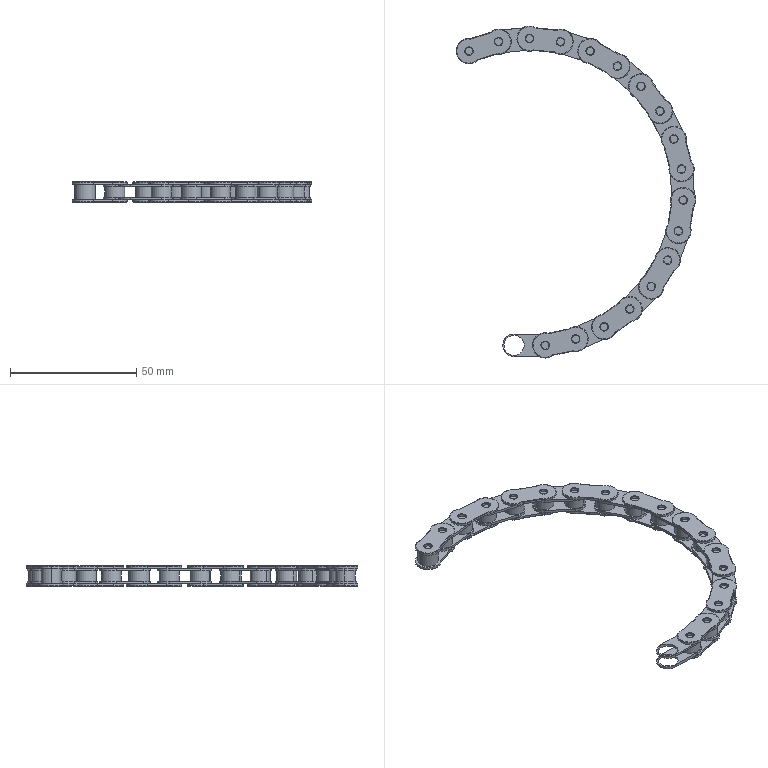Part | STEP file | Front Crank Chain v2 | 9 solids | 594 faces | box 94.978 x 131.686 x 8 mm | volume 9964 mm3 | cylinder 288 | plane 180 | torus 126 | commonest cylinder face diameters 3 x72 8 x72 9 x54 10 x54 0.4 x36